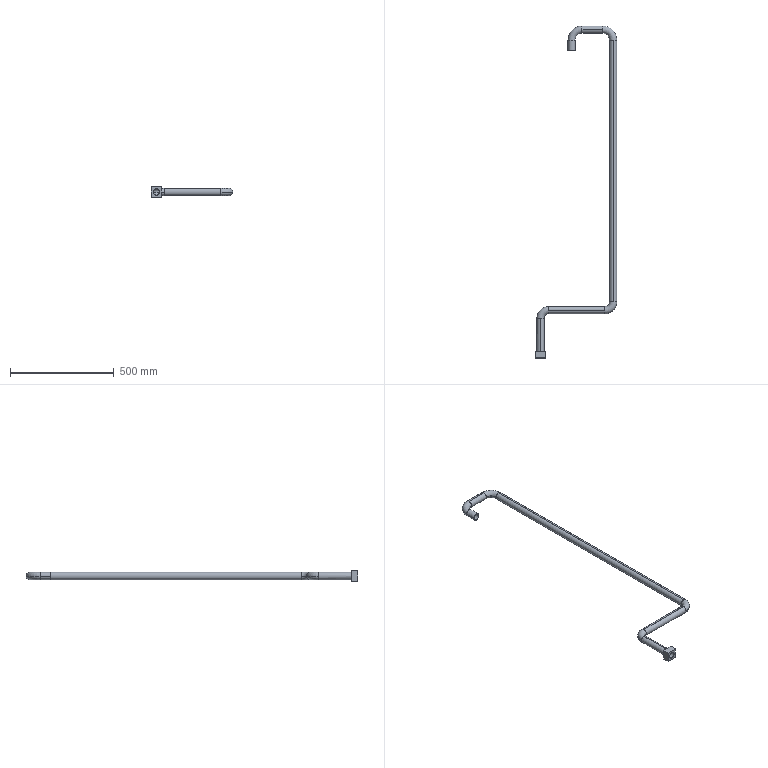Part | STEP file | Water inlet pipe | 1 solid | 43 faces | box 392.5 x 1598 x 50 mm | volume 595634 mm3 | cylinder 20 | torus 16 | plane 7 | commonest cylinder face diameters 30 x10 35 x10